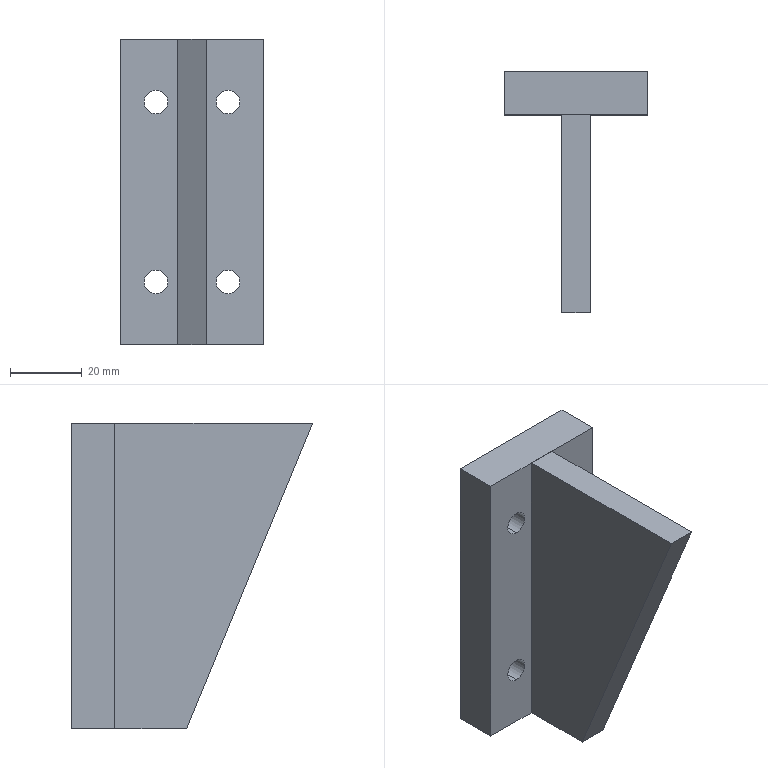Part | STEP file | 01-Positioning block seat | 2 solids | 20 faces | box 40 x 67 x 85 mm | volume 64658 mm3 | plane 12 | cylinder 8 | commonest cylinder face diameters 6.6 x8
STEP:
#1=CARTESIAN_POINT('',(0.,0.,0.));
#2=DIRECTION('',(0.,0.,1.));
#3=DIRECTION('',(1.,0.,0.));
#4=AXIS2_PLACEMENT_3D('',#1,#2,#3);
#5=CARTESIAN_POINT('',(-10.,0.,20.8));
#6=VERTEX_POINT('',#5);
#7=CARTESIAN_POINT('',(-10.,12.,20.8));
#8=VERTEX_POINT('',#7);
#9=CARTESIAN_POINT('',(-10.,27.,20.8));
#10=DIRECTION('',(0.,1.,0.));
#11=VECTOR('',#10,1.);
#12=LINE('',#9,#11);
#13=CARTESIAN_POINT('',(-10.,27.,17.5));
#14=DIRECTION('',(0.,1.,0.));
#15=DIRECTION('',(0.,0.,1.));
#16=AXIS2_PLACEMENT_3D('',#13,#14,#15);
#17=CYLINDRICAL_SURFACE('',#16,3.3);
#18=CARTESIAN_POINT('',(6.283,0.));
#19=DIRECTION('',(0.,1.));
#20=VECTOR('',#19,1.);
#21=LINE('',#18,#20);
#22=(GEOMETRIC_REPRESENTATION_CONTEXT(2)PARAMETRIC_REPRESENTATION_CONTEXT()REPRESENTATION_CONTEXT('',''));
#23=DEFINITIONAL_REPRESENTATION('',(#21),#22);
#24=PCURVE('',#17,#23);
#25=CARTESIAN_POINT('',(-10.,27.,17.5));
#26=DIRECTION('',(0.,1.,0.));
#27=DIRECTION('',(0.,0.,1.));
#28=AXIS2_PLACEMENT_3D('',#25,#26,#27);
#29=CYLINDRICAL_SURFACE('',#28,3.3);
#30=CARTESIAN_POINT('',(0.,0.));
#31=DIRECTION('',(0.,1.));
#32=VECTOR('',#31,1.);
#33=LINE('',#30,#32);
#34=(GEOMETRIC_REPRESENTATION_CONTEXT(2)PARAMETRIC_REPRESENTATION_CONTEXT()REPRESENTATION_CONTEXT('',''));
#35=DEFINITIONAL_REPRESENTATION('',(#33),#34);
#36=PCURVE('',#29,#35);
#37=SURFACE_CURVE('',#12,(#24,#36),.PCURVE_S1.);
#38=EDGE_CURVE('',#6,#8,#37,.T.);
#39=ORIENTED_EDGE('',*,*,#38,.T.);
#40=CARTESIAN_POINT('',(-10.,12.,14.2));
#41=VERTEX_POINT('',#40);
#42=CARTESIAN_POINT('',(-10.,12.,17.5));
#43=DIRECTION('',(0.,-1.,0.));
#44=DIRECTION('',(0.,0.,-1.));
#45=AXIS2_PLACEMENT_3D('',#42,#43,#44);
#46=CIRCLE('',#45,3.3);
#47=CARTESIAN_POINT('',(9.425,-15.));
#48=DIRECTION('',(-1.,0.));
#49=VECTOR('',#48,1.);
#50=LINE('',#47,#49);
#51=(GEOMETRIC_REPRESENTATION_CONTEXT(2)PARAMETRIC_REPRESENTATION_CONTEXT()REPRESENTATION_CONTEXT('',''));
#52=DEFINITIONAL_REPRESENTATION('',(#50),#51);
#53=PCURVE('',#17,#52);
#54=CARTESIAN_POINT('',(20.,12.,85.));
#55=DIRECTION('',(0.,-1.,0.));
#56=DIRECTION('',(0.,0.,-1.));
#57=AXIS2_PLACEMENT_3D('',#54,#55,#56);
#58=PLANE('',#57);
#59=CARTESIAN_POINT('',(67.5,-30.));
#60=DIRECTION('',(1.,0.));
#61=AXIS2_PLACEMENT_2D('',#59,#60);
#62=CIRCLE('',#61,3.3);
#63=(GEOMETRIC_REPRESENTATION_CONTEXT(2)PARAMETRIC_REPRESENTATION_CONTEXT()REPRESENTATION_CONTEXT('',''));
#64=DEFINITIONAL_REPRESENTATION('',(#62),#63);
#65=PCURVE('',#58,#64);
#66=SURFACE_CURVE('',#46,(#53,#65),.PCURVE_S1.);
#67=EDGE_CURVE('',#8,#41,#66,.T.);
#68=ORIENTED_EDGE('',*,*,#67,.T.);
#69=CARTESIAN_POINT('',(-10.,0.,14.2));
#70=VERTEX_POINT('',#69);
#71=CARTESIAN_POINT('',(-10.,27.,14.2));
#72=DIRECTION('',(0.,1.,0.));
#73=VECTOR('',#72,1.);
#74=LINE('',#71,#73);
#75=CARTESIAN_POINT('',(3.142,0.));
#76=DIRECTION('',(0.,1.));
#77=VECTOR('',#76,1.);
#78=LINE('',#75,#77);
#79=(GEOMETRIC_REPRESENTATION_CONTEXT(2)PARAMETRIC_REPRESENTATION_CONTEXT()REPRESENTATION_CONTEXT('',''));
#80=DEFINITIONAL_REPRESENTATION('',(#78),#79);
#81=PCURVE('',#17,#80);
#82=CARTESIAN_POINT('',(3.142,0.));
#83=DIRECTION('',(0.,1.));
#84=VECTOR('',#83,1.);
#85=LINE('',#82,#84);
#86=(GEOMETRIC_REPRESENTATION_CONTEXT(2)PARAMETRIC_REPRESENTATION_CONTEXT()REPRESENTATION_CONTEXT('',''));
#87=DEFINITIONAL_REPRESENTATION('',(#85),#86);
#88=PCURVE('',#29,#87);
#89=SURFACE_CURVE('',#74,(#81,#88),.PCURVE_S1.);
#90=EDGE_CURVE('',#70,#41,#89,.T.);
#91=ORIENTED_EDGE('',*,*,#90,.F.);
#92=CARTESIAN_POINT('',(-10.,0.,17.5));
#93=DIRECTION('',(0.,1.,0.));
#94=DIRECTION('',(0.,0.,1.));
#95=AXIS2_PLACEMENT_3D('',#92,#93,#94);
#96=CIRCLE('',#95,3.3);
#97=CARTESIAN_POINT('',(0.,-27.));
#98=DIRECTION('',(1.,0.));
#99=VECTOR('',#98,1.);
#100=LINE('',#97,#99);
#101=(GEOMETRIC_REPRESENTATION_CONTEXT(2)PARAMETRIC_REPRESENTATION_CONTEXT()REPRESENTATION_CONTEXT('',''));
#102=DEFINITIONAL_REPRESENTATION('',(#100),#101);
#103=PCURVE('',#17,#102);
#104=CARTESIAN_POINT('',(20.,0.,85.));
#105=DIRECTION('',(0.,1.,0.));
#106=DIRECTION('',(0.,0.,1.));
#107=AXIS2_PLACEMENT_3D('',#104,#105,#106);
#108=PLANE('',#107);
#109=CARTESIAN_POINT('',(-67.5,-30.));
#110=DIRECTION('',(1.,0.));
#111=AXIS2_PLACEMENT_2D('',#109,#110);
#112=CIRCLE('',#111,3.3);
#113=(GEOMETRIC_REPRESENTATION_CONTEXT(2)PARAMETRIC_REPRESENTATION_CONTEXT()REPRESENTATION_CONTEXT('',''));
#114=DEFINITIONAL_REPRESENTATION('',(#112),#113);
#115=PCURVE('',#108,#114);
#116=SURFACE_CURVE('',#96,(#103,#115),.PCURVE_S1.);
#117=EDGE_CURVE('',#70,#6,#116,.T.);
#118=ORIENTED_EDGE('',*,*,#117,.T.);
#119=EDGE_LOOP('',(#39,#68,#91,#118));
#120=FACE_BOUND('',#119,.F.);
#121=ADVANCED_FACE('',(#120),#17,.F.);
#122=CARTESIAN_POINT('',(-10.,0.,70.8));
#123=VERTEX_POINT('',#122);
#124=CARTESIAN_POINT('',(-10.,12.,70.8));
#125=VERTEX_POINT('',#124);
#126=CARTESIAN_POINT('',(-10.,27.,70.8));
#127=DIRECTION('',(0.,1.,0.));
#128=VECTOR('',#127,1.);
#129=LINE('',#126,#128);
#130=CARTESIAN_POINT('',(-10.,27.,67.5));
#131=DIRECTION('',(0.,1.,0.));
#132=DIRECTION('',(0.,0.,1.));
#133=AXIS2_PLACEMENT_3D('',#130,#131,#132);
#134=CYLINDRICAL_SURFACE('',#133,3.3);
#135=CARTESIAN_POINT('',(6.283,0.));
#136=DIRECTION('',(0.,1.));
#137=VECTOR('',#136,1.);
#138=LINE('',#135,#137);
#139=(GEOMETRIC_REPRESENTATION_CONTEXT(2)PARAMETRIC_REPRESENTATION_CONTEXT()REPRESENTATION_CONTEXT('',''));
#140=DEFINITIONAL_REPRESENTATION('',(#138),#139);
#141=PCURVE('',#134,#140);
#142=CARTESIAN_POINT('',(-10.,27.,67.5));
#143=DIRECTION('',(0.,1.,0.));
#144=DIRECTION('',(0.,0.,1.));
#145=AXIS2_PLACEMENT_3D('',#142,#143,#144);
#146=CYLINDRICAL_SURFACE('',#145,3.3);
#147=CARTESIAN_POINT('',(0.,0.));
#148=DIRECTION('',(0.,1.));
#149=VECTOR('',#148,1.);
#150=LINE('',#147,#149);
#151=(GEOMETRIC_REPRESENTATION_CONTEXT(2)PARAMETRIC_REPRESENTATION_CONTEXT()REPRESENTATION_CONTEXT('',''));
#152=DEFINITIONAL_REPRESENTATION('',(#150),#151);
#153=PCURVE('',#146,#152);
#154=SURFACE_CURVE('',#129,(#141,#153),.PCURVE_S1.);
#155=EDGE_CURVE('',#123,#125,#154,.T.);
#156=ORIENTED_EDGE('',*,*,#155,.T.);
#157=CARTESIAN_POINT('',(-10.,12.,64.2));
#158=VERTEX_POINT('',#157);
#159=CARTESIAN_POINT('',(-10.,12.,67.5));
#160=DIRECTION('',(0.,-1.,0.));
#161=DIRECTION('',(0.,0.,-1.));
#162=AXIS2_PLACEMENT_3D('',#159,#160,#161);
#163=CIRCLE('',#162,3.3);
#164=CARTESIAN_POINT('',(9.425,-15.));
#165=DIRECTION('',(-1.,0.));
#166=VECTOR('',#165,1.);
#167=LINE('',#164,#166);
#168=(GEOMETRIC_REPRESENTATION_CONTEXT(2)PARAMETRIC_REPRESENTATION_CONTEXT()REPRESENTATION_CONTEXT('',''));
#169=DEFINITIONAL_REPRESENTATION('',(#167),#168);
#170=PCURVE('',#134,#169);
#171=CARTESIAN_POINT('',(17.5,-30.));
#172=DIRECTION('',(1.,0.));
#173=AXIS2_PLACEMENT_2D('',#171,#172);
#174=CIRCLE('',#173,3.3);
#175=(GEOMETRIC_REPRESENTATION_CONTEXT(2)PARAMETRIC_REPRESENTATION_CONTEXT()REPRESENTATION_CONTEXT('',''));
#176=DEFINITIONAL_REPRESENTATION('',(#174),#175);
#177=PCURVE('',#58,#176);
#178=SURFACE_CURVE('',#163,(#170,#177),.PCURVE_S1.);
#179=EDGE_CURVE('',#125,#158,#178,.T.);
#180=ORIENTED_EDGE('',*,*,#179,.T.);
#181=CARTESIAN_POINT('',(-10.,0.,64.2));
#182=VERTEX_POINT('',#181);
#183=CARTESIAN_POINT('',(-10.,27.,64.2));
#184=DIRECTION('',(0.,1.,0.));
#185=VECTOR('',#184,1.);
#186=LINE('',#183,#185);
#187=CARTESIAN_POINT('',(3.142,0.));
#188=DIRECTION('',(0.,1.));
#189=VECTOR('',#188,1.);
#190=LINE('',#187,#189);
#191=(GEOMETRIC_REPRESENTATION_CONTEXT(2)PARAMETRIC_REPRESENTATION_CONTEXT()REPRESENTATION_CONTEXT('',''));
#192=DEFINITIONAL_REPRESENTATION('',(#190),#191);
#193=PCURVE('',#134,#192);
#194=CARTESIAN_POINT('',(3.142,0.));
#195=DIRECTION('',(0.,1.));
#196=VECTOR('',#195,1.);
#197=LINE('',#194,#196);
#198=(GEOMETRIC_REPRESENTATION_CONTEXT(2)PARAMETRIC_REPRESENTATION_CONTEXT()REPRESENTATION_CONTEXT('',''));
#199=DEFINITIONAL_REPRESENTATION('',(#197),#198);
#200=PCURVE('',#146,#199);
#201=SURFACE_CURVE('',#186,(#193,#200),.PCURVE_S1.);
#202=EDGE_CURVE('',#182,#158,#201,.T.);
#203=ORIENTED_EDGE('',*,*,#202,.F.);
#204=CARTESIAN_POINT('',(-10.,0.,67.5));
#205=DIRECTION('',(0.,1.,0.));
#206=DIRECTION('',(0.,0.,1.));
#207=AXIS2_PLACEMENT_3D('',#204,#205,#206);
#208=CIRCLE('',#207,3.3);
#209=CARTESIAN_POINT('',(0.,-27.));
#210=DIRECTION('',(1.,0.));
#211=VECTOR('',#210,1.);
#212=LINE('',#209,#211);
#213=(GEOMETRIC_REPRESENTATION_CONTEXT(2)PARAMETRIC_REPRESENTATION_CONTEXT()REPRESENTATION_CONTEXT('',''));
#214=DEFINITIONAL_REPRESENTATION('',(#212),#213);
#215=PCURVE('',#134,#214);
#216=CARTESIAN_POINT('',(-17.5,-30.));
#217=DIRECTION('',(1.,0.));
#218=AXIS2_PLACEMENT_2D('',#216,#217);
#219=CIRCLE('',#218,3.3);
#220=(GEOMETRIC_REPRESENTATION_CONTEXT(2)PARAMETRIC_REPRESENTATION_CONTEXT()REPRESENTATION_CONTEXT('',''));
#221=DEFINITIONAL_REPRESENTATION('',(#219),#220);
#222=PCURVE('',#108,#221);
#223=SURFACE_CURVE('',#208,(#215,#222),.PCURVE_S1.);
#224=EDGE_CURVE('',#182,#123,#223,.T.);
#225=ORIENTED_EDGE('',*,*,#224,.T.);
#226=EDGE_LOOP('',(#156,#180,#203,#225));
#227=FACE_BOUND('',#226,.F.);
#228=ADVANCED_FACE('',(#227),#134,.F.);
#229=CARTESIAN_POINT('',(10.,0.,20.8));
#230=VERTEX_POINT('',#229);
#231=CARTESIAN_POINT('',(10.,12.,20.8));
#232=VERTEX_POINT('',#231);
#233=CARTESIAN_POINT('',(10.,27.,20.8));
#234=DIRECTION('',(0.,1.,0.));
#235=VECTOR('',#234,1.);
#236=LINE('',#233,#235);
#237=CARTESIAN_POINT('',(10.,27.,17.5));
#238=DIRECTION('',(0.,1.,0.));
#239=DIRECTION('',(0.,0.,1.));
#240=AXIS2_PLACEMENT_3D('',#237,#238,#239);
#241=CYLINDRICAL_SURFACE('',#240,3.3);
#242=CARTESIAN_POINT('',(6.283,0.));
#243=DIRECTION('',(0.,1.));
#244=VECTOR('',#243,1.);
#245=LINE('',#242,#244);
#246=(GEOMETRIC_REPRESENTATION_CONTEXT(2)PARAMETRIC_REPRESENTATION_CONTEXT()REPRESENTATION_CONTEXT('',''));
#247=DEFINITIONAL_REPRESENTATION('',(#245),#246);
#248=PCURVE('',#241,#247);
#249=CARTESIAN_POINT('',(10.,27.,17.5));
#250=DIRECTION('',(0.,1.,0.));
#251=DIRECTION('',(0.,0.,1.));
#252=AXIS2_PLACEMENT_3D('',#249,#250,#251);
#253=CYLINDRICAL_SURFACE('',#252,3.3);
#254=CARTESIAN_POINT('',(0.,0.));
#255=DIRECTION('',(0.,1.));
#256=VECTOR('',#255,1.);
#257=LINE('',#254,#256);
#258=(GEOMETRIC_REPRESENTATION_CONTEXT(2)PARAMETRIC_REPRESENTATION_CONTEXT()REPRESENTATION_CONTEXT('',''));
#259=DEFINITIONAL_REPRESENTATION('',(#257),#258);
#260=PCURVE('',#253,#259);
#261=SURFACE_CURVE('',#236,(#248,#260),.PCURVE_S1.);
#262=EDGE_CURVE('',#230,#232,#261,.T.);
#263=ORIENTED_EDGE('',*,*,#262,.T.);
#264=CARTESIAN_POINT('',(10.,12.,14.2));
#265=VERTEX_POINT('',#264);
#266=CARTESIAN_POINT('',(10.,12.,17.5));
#267=DIRECTION('',(0.,-1.,0.));
#268=DIRECTION('',(0.,0.,-1.));
#269=AXIS2_PLACEMENT_3D('',#266,#267,#268);
#270=CIRCLE('',#269,3.3);
#271=CARTESIAN_POINT('',(9.425,-15.));
#272=DIRECTION('',(-1.,0.));
#273=VECTOR('',#272,1.);
#274=LINE('',#271,#273);
#275=(GEOMETRIC_REPRESENTATION_CONTEXT(2)PARAMETRIC_REPRESENTATION_CONTEXT()REPRESENTATION_CONTEXT('',''));
#276=DEFINITIONAL_REPRESENTATION('',(#274),#275);
#277=PCURVE('',#241,#276);
#278=CARTESIAN_POINT('',(67.5,-10.));
#279=DIRECTION('',(1.,0.));
#280=AXIS2_PLACEMENT_2D('',#278,#279);
#281=CIRCLE('',#280,3.3);
#282=(GEOMETRIC_REPRESENTATION_CONTEXT(2)PARAMETRIC_REPRESENTATION_CONTEXT()REPRESENTATION_CONTEXT('',''));
#283=DEFINITIONAL_REPRESENTATION('',(#281),#282);
#284=PCURVE('',#58,#283);
#285=SURFACE_CURVE('',#270,(#277,#284),.PCURVE_S1.);
#286=EDGE_CURVE('',#232,#265,#285,.T.);
#287=ORIENTED_EDGE('',*,*,#286,.T.);
#288=CARTESIAN_POINT('',(10.,0.,14.2));
#289=VERTEX_POINT('',#288);
#290=CARTESIAN_POINT('',(10.,27.,14.2));
#291=DIRECTION('',(0.,1.,0.));
#292=VECTOR('',#291,1.);
#293=LINE('',#290,#292);
#294=CARTESIAN_POINT('',(3.142,0.));
#295=DIRECTION('',(0.,1.));
#296=VECTOR('',#295,1.);
#297=LINE('',#294,#296);
#298=(GEOMETRIC_REPRESENTATION_CONTEXT(2)PARAMETRIC_REPRESENTATION_CONTEXT()REPRESENTATION_CONTEXT('',''));
#299=DEFINITIONAL_REPRESENTATION('',(#297),#298);
#300=PCURVE('',#241,#299);
#301=CARTESIAN_POINT('',(3.142,0.));
#302=DIRECTION('',(0.,1.));
#303=VECTOR('',#302,1.);
#304=LINE('',#301,#303);
#305=(GEOMETRIC_REPRESENTATION_CONTEXT(2)PARAMETRIC_REPRESENTATION_CONTEXT()REPRESENTATION_CONTEXT('',''));
#306=DEFINITIONAL_REPRESENTATION('',(#304),#305);
#307=PCURVE('',#253,#306);
#308=SURFACE_CURVE('',#293,(#300,#307),.PCURVE_S1.);
#309=EDGE_CURVE('',#289,#265,#308,.T.);
#310=ORIENTED_EDGE('',*,*,#309,.F.);
#311=CARTESIAN_POINT('',(10.,0.,17.5));
#312=DIRECTION('',(0.,1.,0.));
#313=DIRECTION('',(0.,0.,1.));
#314=AXIS2_PLACEMENT_3D('',#311,#312,#313);
#315=CIRCLE('',#314,3.3);
#316=CARTESIAN_POINT('',(0.,-27.));
#317=DIRECTION('',(1.,0.));
#318=VECTOR('',#317,1.);
#319=LINE('',#316,#318);
#320=(GEOMETRIC_REPRESENTATION_CONTEXT(2)PARAMETRIC_REPRESENTATION_CONTEXT()REPRESENTATION_CONTEXT('',''));
#321=DEFINITIONAL_REPRESENTATION('',(#319),#320);
#322=PCURVE('',#241,#321);
#323=CARTESIAN_POINT('',(-67.5,-10.));
#324=DIRECTION('',(1.,0.));
#325=AXIS2_PLACEMENT_2D('',#323,#324);
#326=CIRCLE('',#325,3.3);
#327=(GEOMETRIC_REPRESENTATION_CONTEXT(2)PARAMETRIC_REPRESENTATION_CONTEXT()REPRESENTATION_CONTEXT('',''));
#328=DEFINITIONAL_REPRESENTATION('',(#326),#327);
#329=PCURVE('',#108,#328);
#330=SURFACE_CURVE('',#315,(#322,#329),.PCURVE_S1.);
#331=EDGE_CURVE('',#289,#230,#330,.T.);
#332=ORIENTED_EDGE('',*,*,#331,.T.);
#333=EDGE_LOOP('',(#263,#287,#310,#332));
#334=FACE_BOUND('',#333,.F.);
#335=ADVANCED_FACE('',(#334),#241,.F.);
#336=CARTESIAN_POINT('',(10.,0.,70.8));
#337=VERTEX_POINT('',#336);
#338=CARTESIAN_POINT('',(10.,12.,70.8));
#339=VERTEX_POINT('',#338);
#340=CARTESIAN_POINT('',(10.,27.,70.8));
#341=DIRECTION('',(0.,1.,0.));
#342=VECTOR('',#341,1.);
#343=LINE('',#340,#342);
#344=CARTESIAN_POINT('',(10.,27.,67.5));
#345=DIRECTION('',(0.,1.,0.));
#346=DIRECTION('',(0.,0.,1.));
#347=AXIS2_PLACEMENT_3D('',#344,#345,#346);
#348=CYLINDRICAL_SURFACE('',#347,3.3);
#349=CARTESIAN_POINT('',(6.283,0.));
#350=DIRECTION('',(0.,1.));
#351=VECTOR('',#350,1.);
#352=LINE('',#349,#351);
#353=(GEOMETRIC_REPRESENTATION_CONTEXT(2)PARAMETRIC_REPRESENTATION_CONTEXT()REPRESENTATION_CONTEXT('',''));
#354=DEFINITIONAL_REPRESENTATION('',(#352),#353);
#355=PCURVE('',#348,#354);
#356=CARTESIAN_POINT('',(10.,27.,67.5));
#357=DIRECTION('',(0.,1.,0.));
#358=DIRECTION('',(0.,0.,1.));
#359=AXIS2_PLACEMENT_3D('',#356,#357,#358);
#360=CYLINDRICAL_SURFACE('',#359,3.3);
#361=CARTESIAN_POINT('',(0.,0.));
#362=DIRECTION('',(0.,1.));
#363=VECTOR('',#362,1.);
#364=LINE('',#361,#363);
#365=(GEOMETRIC_REPRESENTATION_CONTEXT(2)PARAMETRIC_REPRESENTATION_CONTEXT()REPRESENTATION_CONTEXT('',''));
#366=DEFINITIONAL_REPRESENTATION('',(#364),#365);
#367=PCURVE('',#360,#366);
#368=SURFACE_CURVE('',#343,(#355,#367),.PCURVE_S1.);
#369=EDGE_CURVE('',#337,#339,#368,.T.);
#370=ORIENTED_EDGE('',*,*,#369,.T.);
#371=CARTESIAN_POINT('',(10.,12.,64.2));
#372=VERTEX_POINT('',#371);
#373=CARTESIAN_POINT('',(10.,12.,67.5));
#374=DIRECTION('',(0.,-1.,0.));
#375=DIRECTION('',(0.,0.,-1.));
#376=AXIS2_PLACEMENT_3D('',#373,#374,#375);
#377=CIRCLE('',#376,3.3);
#378=CARTESIAN_POINT('',(9.425,-15.));
#379=DIRECTION('',(-1.,0.));
#380=VECTOR('',#379,1.);
#381=LINE('',#378,#380);
#382=(GEOMETRIC_REPRESENTATION_CONTEXT(2)PARAMETRIC_REPRESENTATION_CONTEXT()REPRESENTATION_CONTEXT('',''));
#383=DEFINITIONAL_REPRESENTATION('',(#381),#382);
#384=PCURVE('',#348,#383);
#385=CARTESIAN_POINT('',(17.5,-10.));
#386=DIRECTION('',(1.,0.));
#387=AXIS2_PLACEMENT_2D('',#385,#386);
#388=CIRCLE('',#387,3.3);
#389=(GEOMETRIC_REPRESENTATION_CONTEXT(2)PARAMETRIC_REPRESENTATION_CONTEXT()REPRESENTATION_CONTEXT('',''));
#390=DEFINITIONAL_REPRESENTATION('',(#388),#389);
#391=PCURVE('',#58,#390);
#392=SURFACE_CURVE('',#377,(#384,#391),.PCURVE_S1.);
#393=EDGE_CURVE('',#339,#372,#392,.T.);
#394=ORIENTED_EDGE('',*,*,#393,.T.);
#395=CARTESIAN_POINT('',(10.,0.,64.2));
#396=VERTEX_POINT('',#395);
#397=CARTESIAN_POINT('',(10.,27.,64.2));
#398=DIRECTION('',(0.,1.,0.));
#399=VECTOR('',#398,1.);
#400=LINE('',#397,#399);
#401=CARTESIAN_POINT('',(3.142,0.));
#402=DIRECTION('',(0.,1.));
#403=VECTOR('',#402,1.);
#404=LINE('',#401,#403);
#405=(GEOMETRIC_REPRESENTATION_CONTEXT(2)PARAMETRIC_REPRESENTATION_CONTEXT()REPRESENTATION_CONTEXT('',''));
#406=DEFINITIONAL_REPRESENTATION('',(#404),#405);
#407=PCURVE('',#348,#406);
#408=CARTESIAN_POINT('',(3.142,0.));
#409=DIRECTION('',(0.,1.));
#410=VECTOR('',#409,1.);
#411=LINE('',#408,#410);
#412=(GEOMETRIC_REPRESENTATION_CONTEXT(2)PARAMETRIC_REPRESENTATION_CONTEXT()REPRESENTATION_CONTEXT('',''));
#413=DEFINITIONAL_REPRESENTATION('',(#411),#412);
#414=PCURVE('',#360,#413);
#415=SURFACE_CURVE('',#400,(#407,#414),.PCURVE_S1.);
#416=EDGE_CURVE('',#396,#372,#415,.T.);
#417=ORIENTED_EDGE('',*,*,#416,.F.);
#418=CARTESIAN_POINT('',(10.,0.,67.5));
#419=DIRECTION('',(0.,1.,0.));
#420=DIRECTION('',(0.,0.,1.));
#421=AXIS2_PLACEMENT_3D('',#418,#419,#420);
#422=CIRCLE('',#421,3.3);
#423=CARTESIAN_POINT('',(0.,-27.));
#424=DIRECTION('',(1.,0.));
#425=VECTOR('',#424,1.);
#426=LINE('',#423,#425);
#427=(GEOMETRIC_REPRESENTATION_CONTEXT(2)PARAMETRIC_REPRESENTATION_CONTEXT()REPRESENTATION_CONTEXT('',''));
#428=DEFINITIONAL_REPRESENTATION('',(#426),#427);
#429=PCURVE('',#348,#428);
#430=CARTESIAN_POINT('',(-17.5,-10.));
#431=DIRECTION('',(1.,0.));
#432=AXIS2_PLACEMENT_2D('',#430,#431);
#433=CIRCLE('',#432,3.3);
#434=(GEOMETRIC_REPRESENTATION_CONTEXT(2)PARAMETRIC_REPRESENTATION_CONTEXT()REPRESENTATION_CONTEXT('',''));
#435=DEFINITIONAL_REPRESENTATION('',(#433),#434);
#436=PCURVE('',#108,#435);
#437=SURFACE_CURVE('',#422,(#429,#436),.PCURVE_S1.);
#438=EDGE_CURVE('',#396,#337,#437,.T.);
#439=ORIENTED_EDGE('',*,*,#438,.T.);
#440=EDGE_LOOP('',(#370,#394,#417,#439));
#441=FACE_BOUND('',#440,.F.);
#442=ADVANCED_FACE('',(#441),#348,.F.);
#443=CARTESIAN_POINT('',(-20.,12.,85.));
#444=VERTEX_POINT('',#443);
#445=CARTESIAN_POINT('',(-20.,0.,85.));
#446=VERTEX_POINT('',#445);
#447=CARTESIAN_POINT('',(-20.,0.,85.));
#448=DIRECTION('',(0.,-1.,0.));
#449=VECTOR('',#448,1.);
#450=LINE('',#447,#449);
#451=CARTESIAN_POINT('',(20.,0.,85.));
#452=DIRECTION('',(0.,0.,-1.));
#453=DIRECTION('',(-1.,0.,0.));
#454=AXIS2_PLACEMENT_3D('',#451,#452,#453);
#455=PLANE('',#454);
#456=CARTESIAN_POINT('',(40.,0.));
#457=DIRECTION('',(0.,-1.));
#458=VECTOR('',#457,1.);
#459=LINE('',#456,#458);
#460=(GEOMETRIC_REPRESENTATION_CONTEXT(2)PARAMETRIC_REPRESENTATION_CONTEXT()REPRESENTATION_CONTEXT('',''));
#461=DEFINITIONAL_REPRESENTATION('',(#459),#460);
#462=PCURVE('',#455,#461);
#463=CARTESIAN_POINT('',(-20.,0.,0.));
#464=DIRECTION('',(-1.,0.,0.));
#465=DIRECTION('',(0.,0.,1.));
#466=AXIS2_PLACEMENT_3D('',#463,#464,#465);
#467=PLANE('',#466);
#468=CARTESIAN_POINT('',(85.,0.));
#469=DIRECTION('',(0.,-1.));
#470=VECTOR('',#469,1.);
#471=LINE('',#468,#470);
#472=(GEOMETRIC_REPRESENTATION_CONTEXT(2)PARAMETRIC_REPRESENTATION_CONTEXT()REPRESENTATION_CONTEXT('',''));
#473=DEFINITIONAL_REPRESENTATION('',(#471),#472);
#474=PCURVE('',#467,#473);
#475=SURFACE_CURVE('',#450,(#462,#474),.PCURVE_S1.);
#476=EDGE_CURVE('',#444,#446,#475,.T.);
#477=ORIENTED_EDGE('',*,*,#476,.T.);
#478=CARTESIAN_POINT('',(20.,0.,85.));
#479=VERTEX_POINT('',#478);
#480=CARTESIAN_POINT('',(20.,0.,85.));
#481=DIRECTION('',(-1.,0.,0.));
#482=VECTOR('',#481,1.);
#483=LINE('',#480,#482);
#484=CARTESIAN_POINT('',(0.,0.));
#485=DIRECTION('',(1.,0.));
#486=VECTOR('',#485,1.);
#487=LINE('',#484,#486);
#488=(GEOMETRIC_REPRESENTATION_CONTEXT(2)PARAMETRIC_REPRESENTATION_CONTEXT()REPRESENTATION_CONTEXT('',''));
#489=DEFINITIONAL_REPRESENTATION('',(#487),#488);
#490=PCURVE('',#455,#489);
#491=CARTESIAN_POINT('',(0.,0.));
#492=DIRECTION('',(0.,-1.));
#493=VECTOR('',#492,1.);
#494=LINE('',#491,#493);
#495=(GEOMETRIC_REPRESENTATION_CONTEXT(2)PARAMETRIC_REPRESENTATION_CONTEXT()REPRESENTATION_CONTEXT('',''));
#496=DEFINITIONAL_REPRESENTATION('',(#494),#495);
#497=PCURVE('',#108,#496);
#498=SURFACE_CURVE('',#483,(#490,#497),.PCURVE_S1.);
#499=EDGE_CURVE('',#479,#446,#498,.T.);
#500=ORIENTED_EDGE('',*,*,#499,.F.);
#501=CARTESIAN_POINT('',(20.,12.,85.));
#502=VERTEX_POINT('',#501);
#503=CARTESIAN_POINT('',(20.,0.,85.));
#504=DIRECTION('',(0.,-1.,0.));
#505=VECTOR('',#504,1.);
#506=LINE('',#503,#505);
#507=CARTESIAN_POINT('',(0.,0.));
#508=DIRECTION('',(0.,-1.));
#509=VECTOR('',#508,1.);
#510=LINE('',#507,#509);
#511=(GEOMETRIC_REPRESENTATION_CONTEXT(2)PARAMETRIC_REPRESENTATION_CONTEXT()REPRESENTATION_CONTEXT('',''));
#512=DEFINITIONAL_REPRESENTATION('',(#510),#511);
#513=PCURVE('',#455,#512);
#514=CARTESIAN_POINT('',(20.,0.,0.));
#515=DIRECTION('',(-1.,0.,0.));
#516=DIRECTION('',(0.,0.,1.));
#517=AXIS2_PLACEMENT_3D('',#514,#515,#516);
#518=PLANE('',#517);
#519=CARTESIAN_POINT('',(85.,0.));
#520=DIRECTION('',(0.,-1.));
#521=VECTOR('',#520,1.);
#522=LINE('',#519,#521);
#523=(GEOMETRIC_REPRESENTATION_CONTEXT(2)PARAMETRIC_REPRESENTATION_CONTEXT()REPRESENTATION_CONTEXT('',''));
#524=DEFINITIONAL_REPRESENTATION('',(#522),#523);
#525=PCURVE('',#518,#524);
#526=SURFACE_CURVE('',#506,(#513,#525),.PCURVE_S1.);
#527=EDGE_CURVE('',#502,#479,#526,.T.);
#528=ORIENTED_EDGE('',*,*,#527,.F.);
#529=CARTESIAN_POINT('',(20.,12.,85.));
#530=DIRECTION('',(-1.,0.,0.));
#531=VECTOR('',#530,1.);
#532=LINE('',#529,#531);
#533=CARTESIAN_POINT('',(0.,12.));
#534=DIRECTION('',(1.,0.));
#535=VECTOR('',#534,1.);
#536=LINE('',#533,#535);
#537=(GEOMETRIC_REPRESENTATION_CONTEXT(2)PARAMETRIC_REPRESENTATION_CONTEXT()REPRESENTATION_CONTEXT('',''));
#538=DEFINITIONAL_REPRESENTATION('',(#536),#537);
#539=PCURVE('',#455,#538);
#540=CARTESIAN_POINT('',(0.,0.));
#541=DIRECTION('',(0.,-1.));
#542=VECTOR('',#541,1.);
#543=LINE('',#540,#542);
#544=(GEOMETRIC_REPRESENTATION_CONTEXT(2)PARAMETRIC_REPRESENTATION_CONTEXT()REPRESENTATION_CONTEXT('',''));
#545=DEFINITIONAL_REPRESENTATION('',(#543),#544);
#546=PCURVE('',#58,#545);
#547=SURFACE_CURVE('',#532,(#539,#546),.PCURVE_S1.);
#548=EDGE_CURVE('',#502,#444,#547,.T.);
#549=ORIENTED_EDGE('',*,*,#548,.T.);
#550=EDGE_LOOP('',(#477,#500,#528,#549));
#551=FACE_BOUND('',#550,.T.);
#552=ADVANCED_FACE('',(#551),#455,.F.);
#553=CARTESIAN_POINT('',(-10.,0.,17.5));
#554=DIRECTION('',(0.,1.,0.));
#555=DIRECTION('',(0.,0.,1.));
#556=AXIS2_PLACEMENT_3D('',#553,#554,#555);
#557=CIRCLE('',#556,3.3);
#558=CARTESIAN_POINT('',(-67.5,-30.));
#559=DIRECTION('',(1.,0.));
#560=AXIS2_PLACEMENT_2D('',#558,#559);
#561=CIRCLE('',#560,3.3);
#562=(GEOMETRIC_REPRESENTATION_CONTEXT(2)PARAMETRIC_REPRESENTATION_CONTEXT()REPRESENTATION_CONTEXT('',''));
#563=DEFINITIONAL_REPRESENTATION('',(#561),#562);
#564=PCURVE('',#108,#563);
#565=CARTESIAN_POINT('',(0.,-27.));
#566=DIRECTION('',(1.,0.));
#567=VECTOR('',#566,1.);
#568=LINE('',#565,#567);
#569=(GEOMETRIC_REPRESENTATION_CONTEXT(2)PARAMETRIC_REPRESENTATION_CONTEXT()REPRESENTATION_CONTEXT('',''));
#570=DEFINITIONAL_REPRESENTATION('',(#568),#569);
#571=PCURVE('',#29,#570);
#572=SURFACE_CURVE('',#557,(#564,#571),.PCURVE_S1.);
#573=EDGE_CURVE('',#6,#70,#572,.T.);
#574=ORIENTED_EDGE('',*,*,#573,.T.);
#575=ORIENTED_EDGE('',*,*,#117,.T.);
#576=EDGE_LOOP('',(#574,#575));
#577=FACE_BOUND('',#576,.T.);
#578=CARTESIAN_POINT('',(-10.,0.,67.5));
#579=DIRECTION('',(0.,1.,0.));
#580=DIRECTION('',(0.,0.,1.));
#581=AXIS2_PLACEMENT_3D('',#578,#579,#580);
#582=CIRCLE('',#581,3.3);
#583=CARTESIAN_POINT('',(-17.5,-30.));
#584=DIRECTION('',(1.,0.));
#585=AXIS2_PLACEMENT_2D('',#583,#584);
#586=CIRCLE('',#585,3.3);
#587=(GEOMETRIC_REPRESENTATION_CONTEXT(2)PARAMETRIC_REPRESENTATION_CONTEXT()REPRESENTATION_CONTEXT('',''));
#588=DEFINITIONAL_REPRESENTATION('',(#586),#587);
#589=PCURVE('',#108,#588);
#590=CARTESIAN_POINT('',(0.,-27.));
#591=DIRECTION('',(1.,0.));
#592=VECTOR('',#591,1.);
#593=LINE('',#590,#592);
#594=(GEOMETRIC_REPRESENTATION_CONTEXT(2)PARAMETRIC_REPRESENTATION_CONTEXT()REPRESENTATION_CONTEXT('',''));
#595=DEFINITIONAL_REPRESENTATION('',(#593),#594);
#596=PCURVE('',#146,#595);
#597=SURFACE_CURVE('',#582,(#589,#596),.PCURVE_S1.);
#598=EDGE_CURVE('',#123,#182,#597,.T.);
#599=ORIENTED_EDGE('',*,*,#598,.T.);
#600=ORIENTED_EDGE('',*,*,#224,.T.);
#601=EDGE_LOOP('',(#599,#600));
#602=FACE_BOUND('',#601,.T.);
#603=CARTESIAN_POINT('',(10.,0.,17.5));
#604=DIRECTION('',(0.,1.,0.));
#605=DIRECTION('',(0.,0.,1.));
#606=AXIS2_PLACEMENT_3D('',#603,#604,#605);
#607=CIRCLE('',#606,3.3);
#608=CARTESIAN_POINT('',(-67.5,-10.));
#609=DIRECTION('',(1.,0.));
#610=AXIS2_PLACEMENT_2D('',#608,#609);
#611=CIRCLE('',#610,3.3);
#612=(GEOMETRIC_REPRESENTATION_CONTEXT(2)PARAMETRIC_REPRESENTATION_CONTEXT()REPRESENTATION_CONTEXT('',''));
#613=DEFINITIONAL_REPRESENTATION('',(#611),#612);
#614=PCURVE('',#108,#613);
#615=CARTESIAN_POINT('',(0.,-27.));
#616=DIRECTION('',(1.,0.));
#617=VECTOR('',#616,1.);
#618=LINE('',#615,#617);
#619=(GEOMETRIC_REPRESENTATION_CONTEXT(2)PARAMETRIC_REPRESENTATION_CONTEXT()REPRESENTATION_CONTEXT('',''));
#620=DEFINITIONAL_REPRESENTATION('',(#618),#619);
#621=PCURVE('',#253,#620);
#622=SURFACE_CURVE('',#607,(#614,#621),.PCURVE_S1.);
#623=EDGE_CURVE('',#230,#289,#622,.T.);
#624=ORIENTED_EDGE('',*,*,#623,.T.);
#625=ORIENTED_EDGE('',*,*,#331,.T.);
#626=EDGE_LOOP('',(#624,#625));
#627=FACE_BOUND('',#626,.T.);
#628=CARTESIAN_POINT('',(10.,0.,67.5));
#629=DIRECTION('',(0.,1.,0.));
#630=DIRECTION('',(0.,0.,1.));
#631=AXIS2_PLACEMENT_3D('',#628,#629,#630);
#632=CIRCLE('',#631,3.3);
#633=CARTESIAN_POINT('',(-17.5,-10.));
#634=DIRECTION('',(1.,0.));
#635=AXIS2_PLACEMENT_2D('',#633,#634);
#636=CIRCLE('',#635,3.3);
#637=(GEOMETRIC_REPRESENTATION_CONTEXT(2)PARAMETRIC_REPRESENTATION_CONTEXT()REPRESENTATION_CONTEXT('',''));
#638=DEFINITIONAL_REPRESENTATION('',(#636),#637);
#639=PCURVE('',#108,#638);
#640=CARTESIAN_POINT('',(0.,-27.));
#641=DIRECTION('',(1.,0.));
#642=VECTOR('',#641,1.);
#643=LINE('',#640,#642);
#644=(GEOMETRIC_REPRESENTATION_CONTEXT(2)PARAMETRIC_REPRESENTATION_CONTEXT()REPRESENTATION_CONTEXT('',''));
#645=DEFINITIONAL_REPRESENTATION('',(#643),#644);
#646=PCURVE('',#360,#645);
#647=SURFACE_CURVE('',#632,(#639,#646),.PCURVE_S1.);
#648=EDGE_CURVE('',#337,#396,#647,.T.);
#649=ORIENTED_EDGE('',*,*,#648,.T.);
#650=ORIENTED_EDGE('',*,*,#438,.T.);
#651=EDGE_LOOP('',(#649,#650));
#652=FACE_BOUND('',#651,.T.);
#653=CARTESIAN_POINT('',(-20.,0.,0.));
#654=VERTEX_POINT('',#653);
#655=CARTESIAN_POINT('',(-20.,0.,85.));
#656=DIRECTION('',(0.,0.,-1.));
#657=VECTOR('',#656,1.);
#658=LINE('',#655,#657);
#659=CARTESIAN_POINT('',(0.,-40.));
#660=DIRECTION('',(-1.,0.));
#661=VECTOR('',#660,1.);
#662=LINE('',#659,#661);
#663=(GEOMETRIC_REPRESENTATION_CONTEXT(2)PARAMETRIC_REPRESENTATION_CONTEXT()REPRESENTATION_CONTEXT('',''));
#664=DEFINITIONAL_REPRESENTATION('',(#662),#663);
#665=PCURVE('',#108,#664);
#666=CARTESIAN_POINT('',(85.,0.));
#667=DIRECTION('',(-1.,0.));
#668=VECTOR('',#667,1.);
#669=LINE('',#666,#668);
#670=(GEOMETRIC_REPRESENTATION_CONTEXT(2)PARAMETRIC_REPRESENTATION_CONTEXT()REPRESENTATION_CONTEXT('',''));
#671=DEFINITIONAL_REPRESENTATION('',(#669),#670);
#672=PCURVE('',#467,#671);
#673=SURFACE_CURVE('',#658,(#665,#672),.PCURVE_S1.);
#674=EDGE_CURVE('',#446,#654,#673,.T.);
#675=ORIENTED_EDGE('',*,*,#674,.T.);
#676=CARTESIAN_POINT('',(20.,0.,0.));
#677=VERTEX_POINT('',#676);
#678=CARTESIAN_POINT('',(20.,0.,0.));
#679=DIRECTION('',(-1.,0.,0.));
#680=VECTOR('',#679,1.);
#681=LINE('',#678,#680);
#682=CARTESIAN_POINT('',(-85.,0.));
#683=DIRECTION('',(0.,-1.));
#684=VECTOR('',#683,1.);
#685=LINE('',#682,#684);
#686=(GEOMETRIC_REPRESENTATION_CONTEXT(2)PARAMETRIC_REPRESENTATION_CONTEXT()REPRESENTATION_CONTEXT('',''));
#687=DEFINITIONAL_REPRESENTATION('',(#685),#686);
#688=PCURVE('',#108,#687);
#689=CARTESIAN_POINT('',(20.,0.,0.));
#690=DIRECTION('',(0.,0.,1.));
#691=DIRECTION('',(1.,0.,0.));
#692=AXIS2_PLACEMENT_3D('',#689,#690,#691);
#693=PLANE('',#692);
#694=CARTESIAN_POINT('',(0.,0.));
#695=DIRECTION('',(-1.,0.));
#696=VECTOR('',#695,1.);
#697=LINE('',#694,#696);
#698=(GEOMETRIC_REPRESENTATION_CONTEXT(2)PARAMETRIC_REPRESENTATION_CONTEXT()REPRESENTATION_CONTEXT('',''));
#699=DEFINITIONAL_REPRESENTATION('',(#697),#698);
#700=PCURVE('',#693,#699);
#701=SURFACE_CURVE('',#681,(#688,#700),.PCURVE_S1.);
#702=EDGE_CURVE('',#677,#654,#701,.T.);
#703=ORIENTED_EDGE('',*,*,#702,.F.);
#704=CARTESIAN_POINT('',(20.,0.,85.));
#705=DIRECTION('',(0.,0.,-1.));
#706=VECTOR('',#705,1.);
#707=LINE('',#704,#706);
#708=CARTESIAN_POINT('',(0.,0.));
#709=DIRECTION('',(-1.,0.));
#710=VECTOR('',#709,1.);
#711=LINE('',#708,#710);
#712=(GEOMETRIC_REPRESENTATION_CONTEXT(2)PARAMETRIC_REPRESENTATION_CONTEXT()REPRESENTATION_CONTEXT('',''));
#713=DEFINITIONAL_REPRESENTATION('',(#711),#712);
#714=PCURVE('',#108,#713);
#715=CARTESIAN_POINT('',(85.,0.));
#716=DIRECTION('',(-1.,0.));
#717=VECTOR('',#716,1.);
#718=LINE('',#715,#717);
#719=(GEOMETRIC_REPRESENTATION_CONTEXT(2)PARAMETRIC_REPRESENTATION_CONTEXT()REPRESENTATION_CONTEXT('',''));
#720=DEFINITIONAL_REPRESENTATION('',(#718),#719);
#721=PCURVE('',#518,#720);
#722=SURFACE_CURVE('',#707,(#714,#721),.PCURVE_S1.);
#723=EDGE_CURVE('',#479,#677,#722,.T.);
#724=ORIENTED_EDGE('',*,*,#723,.F.);
#725=ORIENTED_EDGE('',*,*,#499,.T.);
#726=EDGE_LOOP('',(#675,#703,#724,#725));
#727=FACE_BOUND('',#726,.T.);
#728=ADVANCED_FACE('',(#577,#602,#627,#652,#727),#108,.F.);
#729=CARTESIAN_POINT('',(-20.,12.,0.));
#730=VERTEX_POINT('',#729);
#731=CARTESIAN_POINT('',(-20.,0.,0.));
#732=DIRECTION('',(0.,1.,0.));
#733=VECTOR('',#732,1.);
#734=LINE('',#731,#733);
#735=CARTESIAN_POINT('',(-40.,0.));
#736=DIRECTION('',(0.,1.));
#737=VECTOR('',#736,1.);
#738=LINE('',#735,#737);
#739=(GEOMETRIC_REPRESENTATION_CONTEXT(2)PARAMETRIC_REPRESENTATION_CONTEXT()REPRESENTATION_CONTEXT('',''));
#740=DEFINITIONAL_REPRESENTATION('',(#738),#739);
#741=PCURVE('',#693,#740);
#742=CARTESIAN_POINT('',(0.,0.));
#743=DIRECTION('',(0.,1.));
#744=VECTOR('',#743,1.);
#745=LINE('',#742,#744);
#746=(GEOMETRIC_REPRESENTATION_CONTEXT(2)PARAMETRIC_REPRESENTATION_CONTEXT()REPRESENTATION_CONTEXT('',''));
#747=DEFINITIONAL_REPRESENTATION('',(#745),#746);
#748=PCURVE('',#467,#747);
#749=SURFACE_CURVE('',#734,(#741,#748),.PCURVE_S1.);
#750=EDGE_CURVE('',#654,#730,#749,.T.);
#751=ORIENTED_EDGE('',*,*,#750,.T.);
#752=CARTESIAN_POINT('',(20.,12.,0.));
#753=VERTEX_POINT('',#752);
#754=CARTESIAN_POINT('',(20.,12.,0.));
#755=DIRECTION('',(-1.,0.,0.));
#756=VECTOR('',#755,1.);
#757=LINE('',#754,#756);
#758=CARTESIAN_POINT('',(0.,12.));
#759=DIRECTION('',(-1.,0.));
#760=VECTOR('',#759,1.);
#761=LINE('',#758,#760);
#762=(GEOMETRIC_REPRESENTATION_CONTEXT(2)PARAMETRIC_REPRESENTATION_CONTEXT()REPRESENTATION_CONTEXT('',''));
#763=DEFINITIONAL_REPRESENTATION('',(#761),#762);
#764=PCURVE('',#693,#763);
#765=CARTESIAN_POINT('',(85.,0.));
#766=DIRECTION('',(0.,-1.));
#767=VECTOR('',#766,1.);
#768=LINE('',#765,#767);
#769=(GEOMETRIC_REPRESENTATION_CONTEXT(2)PARAMETRIC_REPRESENTATION_CONTEXT()REPRESENTATION_CONTEXT('',''));
#770=DEFINITIONAL_REPRESENTATION('',(#768),#769);
#771=PCURVE('',#58,#770);
#772=SURFACE_CURVE('',#757,(#764,#771),.PCURVE_S1.);
#773=EDGE_CURVE('',#753,#730,#772,.T.);
#774=ORIENTED_EDGE('',*,*,#773,.F.);
#775=CARTESIAN_POINT('',(20.,0.,0.));
#776=DIRECTION('',(0.,1.,0.));
#777=VECTOR('',#776,1.);
#778=LINE('',#775,#777);
#779=CARTESIAN_POINT('',(0.,0.));
#780=DIRECTION('',(0.,1.));
#781=VECTOR('',#780,1.);
#782=LINE('',#779,#781);
#783=(GEOMETRIC_REPRESENTATION_CONTEXT(2)PARAMETRIC_REPRESENTATION_CONTEXT()REPRESENTATION_CONTEXT('',''));
#784=DEFINITIONAL_REPRESENTATION('',(#782),#783);
#785=PCURVE('',#693,#784);
#786=CARTESIAN_POINT('',(0.,0.));
#787=DIRECTION('',(0.,1.));
#788=VECTOR('',#787,1.);
#789=LINE('',#786,#788);
#790=(GEOMETRIC_REPRESENTATION_CONTEXT(2)PARAMETRIC_REPRESENTATION_CONTEXT()REPRESENTATION_CONTEXT('',''));
#791=DEFINITIONAL_REPRESENTATION('',(#789),#790);
#792=PCURVE('',#518,#791);
#793=SURFACE_CURVE('',#778,(#785,#792),.PCURVE_S1.);
#794=EDGE_CURVE('',#677,#753,#793,.T.);
#795=ORIENTED_EDGE('',*,*,#794,.F.);
#796=ORIENTED_EDGE('',*,*,#702,.T.);
#797=EDGE_LOOP('',(#751,#774,#795,#796));
#798=FACE_BOUND('',#797,.T.);
#799=ADVANCED_FACE('',(#798),#693,.F.);
#800=ORIENTED_EDGE('',*,*,#67,.T.);
#801=CARTESIAN_POINT('',(-10.,12.,17.5));
#802=DIRECTION('',(0.,-1.,0.));
#803=DIRECTION('',(0.,0.,-1.));
#804=AXIS2_PLACEMENT_3D('',#801,#802,#803);
#805=CIRCLE('',#804,3.3);
#806=CARTESIAN_POINT('',(67.5,-30.));
#807=DIRECTION('',(1.,0.));
#808=AXIS2_PLACEMENT_2D('',#806,#807);
#809=CIRCLE('',#808,3.3);
#810=(GEOMETRIC_REPRESENTATION_CONTEXT(2)PARAMETRIC_REPRESENTATION_CONTEXT()REPRESENTATION_CONTEXT('',''));
#811=DEFINITIONAL_REPRESENTATION('',(#809),#810);
#812=PCURVE('',#58,#811);
#813=CARTESIAN_POINT('',(3.142,-15.));
#814=DIRECTION('',(-1.,0.));
#815=VECTOR('',#814,1.);
#816=LINE('',#813,#815);
#817=(GEOMETRIC_REPRESENTATION_CONTEXT(2)PARAMETRIC_REPRESENTATION_CONTEXT()REPRESENTATION_CONTEXT('',''));
#818=DEFINITIONAL_REPRESENTATION('',(#816),#817);
#819=PCURVE('',#29,#818);
#820=SURFACE_CURVE('',#805,(#812,#819),.PCURVE_S1.);
#821=EDGE_CURVE('',#41,#8,#820,.T.);
#822=ORIENTED_EDGE('',*,*,#821,.T.);
#823=EDGE_LOOP('',(#800,#822));
#824=FACE_BOUND('',#823,.T.);
#825=ORIENTED_EDGE('',*,*,#179,.T.);
#826=CARTESIAN_POINT('',(-10.,12.,67.5));
#827=DIRECTION('',(0.,-1.,0.));
#828=DIRECTION('',(0.,0.,-1.));
#829=AXIS2_PLACEMENT_3D('',#826,#827,#828);
#830=CIRCLE('',#829,3.3);
#831=CARTESIAN_POINT('',(17.5,-30.));
#832=DIRECTION('',(1.,0.));
#833=AXIS2_PLACEMENT_2D('',#831,#832);
#834=CIRCLE('',#833,3.3);
#835=(GEOMETRIC_REPRESENTATION_CONTEXT(2)PARAMETRIC_REPRESENTATION_CONTEXT()REPRESENTATION_CONTEXT('',''));
#836=DEFINITIONAL_REPRESENTATION('',(#834),#835);
#837=PCURVE('',#58,#836);
#838=CARTESIAN_POINT('',(3.142,-15.));
#839=DIRECTION('',(-1.,0.));
#840=VECTOR('',#839,1.);
#841=LINE('',#838,#840);
#842=(GEOMETRIC_REPRESENTATION_CONTEXT(2)PARAMETRIC_REPRESENTATION_CONTEXT()REPRESENTATION_CONTEXT('',''));
#843=DEFINITIONAL_REPRESENTATION('',(#841),#842);
#844=PCURVE('',#146,#843);
#845=SURFACE_CURVE('',#830,(#837,#844),.PCURVE_S1.);
#846=EDGE_CURVE('',#158,#125,#845,.T.);
#847=ORIENTED_EDGE('',*,*,#846,.T.);
#848=EDGE_LOOP('',(#825,#847));
#849=FACE_BOUND('',#848,.T.);
#850=ORIENTED_EDGE('',*,*,#286,.T.);
#851=CARTESIAN_POINT('',(10.,12.,17.5));
#852=DIRECTION('',(0.,-1.,0.));
#853=DIRECTION('',(0.,0.,-1.));
#854=AXIS2_PLACEMENT_3D('',#851,#852,#853);
#855=CIRCLE('',#854,3.3);
#856=CARTESIAN_POINT('',(67.5,-10.));
#857=DIRECTION('',(1.,0.));
#858=AXIS2_PLACEMENT_2D('',#856,#857);
#859=CIRCLE('',#858,3.3);
#860=(GEOMETRIC_REPRESENTATION_CONTEXT(2)PARAMETRIC_REPRESENTATION_CONTEXT()REPRESENTATION_CONTEXT('',''));
#861=DEFINITIONAL_REPRESENTATION('',(#859),#860);
#862=PCURVE('',#58,#861);
#863=CARTESIAN_POINT('',(3.142,-15.));
#864=DIRECTION('',(-1.,0.));
#865=VECTOR('',#864,1.);
#866=LINE('',#863,#865);
#867=(GEOMETRIC_REPRESENTATION_CONTEXT(2)PARAMETRIC_REPRESENTATION_CONTEXT()REPRESENTATION_CONTEXT('',''));
#868=DEFINITIONAL_REPRESENTATION('',(#866),#867);
#869=PCURVE('',#253,#868);
#870=SURFACE_CURVE('',#855,(#862,#869),.PCURVE_S1.);
#871=EDGE_CURVE('',#265,#232,#870,.T.);
#872=ORIENTED_EDGE('',*,*,#871,.T.);
#873=EDGE_LOOP('',(#850,#872));
#874=FACE_BOUND('',#873,.T.);
#875=ORIENTED_EDGE('',*,*,#393,.T.);
#876=CARTESIAN_POINT('',(10.,12.,67.5));
#877=DIRECTION('',(0.,-1.,0.));
#878=DIRECTION('',(0.,0.,-1.));
#879=AXIS2_PLACEMENT_3D('',#876,#877,#878);
#880=CIRCLE('',#879,3.3);
#881=CARTESIAN_POINT('',(17.5,-10.));
#882=DIRECTION('',(1.,0.));
#883=AXIS2_PLACEMENT_2D('',#881,#882);
#884=CIRCLE('',#883,3.3);
#885=(GEOMETRIC_REPRESENTATION_CONTEXT(2)PARAMETRIC_REPRESENTATION_CONTEXT()REPRESENTATION_CONTEXT('',''));
#886=DEFINITIONAL_REPRESENTATION('',(#884),#885);
#887=PCURVE('',#58,#886);
#888=CARTESIAN_POINT('',(3.142,-15.));
#889=DIRECTION('',(-1.,0.));
#890=VECTOR('',#889,1.);
#891=LINE('',#888,#890);
#892=(GEOMETRIC_REPRESENTATION_CONTEXT(2)PARAMETRIC_REPRESENTATION_CONTEXT()REPRESENTATION_CONTEXT('',''));
#893=DEFINITIONAL_REPRESENTATION('',(#891),#892);
#894=PCURVE('',#360,#893);
#895=SURFACE_CURVE('',#880,(#887,#894),.PCURVE_S1.);
#896=EDGE_CURVE('',#372,#339,#895,.T.);
#897=ORIENTED_EDGE('',*,*,#896,.T.);
#898=EDGE_LOOP('',(#875,#897));
#899=FACE_BOUND('',#898,.T.);
#900=CARTESIAN_POINT('',(-20.,12.,85.));
#901=DIRECTION('',(0.,0.,1.));
#902=VECTOR('',#901,1.);
#903=LINE('',#900,#902);
#904=CARTESIAN_POINT('',(0.,-40.));
#905=DIRECTION('',(-1.,0.));
#906=VECTOR('',#905,1.);
#907=LINE('',#904,#906);
#908=(GEOMETRIC_REPRESENTATION_CONTEXT(2)PARAMETRIC_REPRESENTATION_CONTEXT()REPRESENTATION_CONTEXT('',''));
#909=DEFINITIONAL_REPRESENTATION('',(#907),#908);
#910=PCURVE('',#58,#909);
#911=CARTESIAN_POINT('',(85.,12.));
#912=DIRECTION('',(1.,0.));
#913=VECTOR('',#912,1.);
#914=LINE('',#911,#913);
#915=(GEOMETRIC_REPRESENTATION_CONTEXT(2)PARAMETRIC_REPRESENTATION_CONTEXT()REPRESENTATION_CONTEXT('',''));
#916=DEFINITIONAL_REPRESENTATION('',(#914),#915);
#917=PCURVE('',#467,#916);
#918=SURFACE_CURVE('',#903,(#910,#917),.PCURVE_S1.);
#919=EDGE_CURVE('',#730,#444,#918,.T.);
#920=ORIENTED_EDGE('',*,*,#919,.T.);
#921=ORIENTED_EDGE('',*,*,#548,.F.);
#922=CARTESIAN_POINT('',(20.,12.,85.));
#923=DIRECTION('',(0.,0.,1.));
#924=VECTOR('',#923,1.);
#925=LINE('',#922,#924);
#926=CARTESIAN_POINT('',(0.,0.));
#927=DIRECTION('',(-1.,0.));
#928=VECTOR('',#927,1.);
#929=LINE('',#926,#928);
#930=(GEOMETRIC_REPRESENTATION_CONTEXT(2)PARAMETRIC_REPRESENTATION_CONTEXT()REPRESENTATION_CONTEXT('',''));
#931=DEFINITIONAL_REPRESENTATION('',(#929),#930);
#932=PCURVE('',#58,#931);
#933=CARTESIAN_POINT('',(85.,12.));
#934=DIRECTION('',(1.,0.));
#935=VECTOR('',#934,1.);
#936=LINE('',#933,#935);
#937=(GEOMETRIC_REPRESENTATION_CONTEXT(2)PARAMETRIC_REPRESENTATION_CONTEXT()REPRESENTATION_CONTEXT('',''));
#938=DEFINITIONAL_REPRESENTATION('',(#936),#937);
#939=PCURVE('',#518,#938);
#940=SURFACE_CURVE('',#925,(#932,#939),.PCURVE_S1.);
#941=EDGE_CURVE('',#753,#502,#940,.T.);
#942=ORIENTED_EDGE('',*,*,#941,.F.);
#943=ORIENTED_EDGE('',*,*,#773,.T.);
#944=EDGE_LOOP('',(#920,#921,#942,#943));
#945=FACE_BOUND('',#944,.T.);
#946=ADVANCED_FACE('',(#824,#849,#874,#899,#945),#58,.F.);
#947=ORIENTED_EDGE('',*,*,#527,.T.);
#948=ORIENTED_EDGE('',*,*,#723,.T.);
#949=ORIENTED_EDGE('',*,*,#794,.T.);
#950=ORIENTED_EDGE('',*,*,#941,.T.);
#951=EDGE_LOOP('',(#947,#948,#949,#950));
#952=FACE_BOUND('',#951,.T.);
#953=ADVANCED_FACE('',(#952),#518,.F.);
#954=ORIENTED_EDGE('',*,*,#476,.F.);
#955=ORIENTED_EDGE('',*,*,#919,.F.);
#956=ORIENTED_EDGE('',*,*,#750,.F.);
#957=ORIENTED_EDGE('',*,*,#674,.F.);
#958=EDGE_LOOP('',(#954,#955,#956,#957));
#959=FACE_BOUND('',#958,.T.);
#960=ADVANCED_FACE('',(#959),#467,.T.);
#961=ORIENTED_EDGE('',*,*,#896,.T.);
#962=ORIENTED_EDGE('',*,*,#369,.F.);
#963=ORIENTED_EDGE('',*,*,#648,.T.);
#964=ORIENTED_EDGE('',*,*,#416,.T.);
#965=EDGE_LOOP('',(#961,#962,#963,#964));
#966=FACE_BOUND('',#965,.F.);
#967=ADVANCED_FACE('',(#966),#360,.F.);
#968=ORIENTED_EDGE('',*,*,#871,.T.);
#969=ORIENTED_EDGE('',*,*,#262,.F.);
#970=ORIENTED_EDGE('',*,*,#623,.T.);
#971=ORIENTED_EDGE('',*,*,#309,.T.);
#972=EDGE_LOOP('',(#968,#969,#970,#971));
#973=FACE_BOUND('',#972,.F.);
#974=ADVANCED_FACE('',(#973),#253,.F.);
#975=ORIENTED_EDGE('',*,*,#846,.T.);
#976=ORIENTED_EDGE('',*,*,#155,.F.);
#977=ORIENTED_EDGE('',*,*,#598,.T.);
#978=ORIENTED_EDGE('',*,*,#202,.T.);
#979=EDGE_LOOP('',(#975,#976,#977,#978));
#980=FACE_BOUND('',#979,.F.);
#981=ADVANCED_FACE('',(#980),#146,.F.);
#982=ORIENTED_EDGE('',*,*,#821,.T.);
#983=ORIENTED_EDGE('',*,*,#38,.F.);
#984=ORIENTED_EDGE('',*,*,#573,.T.);
#985=ORIENTED_EDGE('',*,*,#90,.T.);
#986=EDGE_LOOP('',(#982,#983,#984,#985));
#987=FACE_BOUND('',#986,.F.);
#988=ADVANCED_FACE('',(#987),#29,.F.);
#989=CLOSED_SHELL('',(#121,#228,#335,#442,#552,#728,#799,#946,#953,#960,#967,#974,#981,#988));
#990=MANIFOLD_SOLID_BREP('',#989);
#991=CARTESIAN_POINT('',(-4.,-20.,0.));
#992=VERTEX_POINT('',#991);
#993=CARTESIAN_POINT('',(-4.,0.,0.));
#994=VERTEX_POINT('',#993);
#995=CARTESIAN_POINT('',(-4.,-20.,0.));
#996=DIRECTION('',(0.,1.,0.));
#997=VECTOR('',#996,1.);
#998=LINE('',#995,#997);
#999=CARTESIAN_POINT('',(4.,-20.,0.));
#1000=DIRECTION('',(0.,0.,1.));
#1001=DIRECTION('',(1.,0.,0.));
#1002=AXIS2_PLACEMENT_3D('',#999,#1000,#1001);
#1003=PLANE('',#1002);
#1004=CARTESIAN_POINT('',(-8.,0.));
#1005=DIRECTION('',(0.,1.));
#1006=VECTOR('',#1005,1.);
#1007=LINE('',#1004,#1006);
#1008=(GEOMETRIC_REPRESENTATION_CONTEXT(2)PARAMETRIC_REPRESENTATION_CONTEXT()REPRESENTATION_CONTEXT('',''));
#1009=DEFINITIONAL_REPRESENTATION('',(#1007),#1008);
#1010=PCURVE('',#1003,#1009);
#1011=CARTESIAN_POINT('',(-4.,0.,0.));
#1012=DIRECTION('',(1.,0.,0.));
#1013=DIRECTION('',(0.,0.,-1.));
#1014=AXIS2_PLACEMENT_3D('',#1011,#1012,#1013);
#1015=PLANE('',#1014);
#1016=CARTESIAN_POINT('',(0.,-20.));
#1017=DIRECTION('',(0.,1.));
#1018=VECTOR('',#1017,1.);
#1019=LINE('',#1016,#1018);
#1020=(GEOMETRIC_REPRESENTATION_CONTEXT(2)PARAMETRIC_REPRESENTATION_CONTEXT()REPRESENTATION_CONTEXT('',''));
#1021=DEFINITIONAL_REPRESENTATION('',(#1019),#1020);
#1022=PCURVE('',#1015,#1021);
#1023=SURFACE_CURVE('',#998,(#1010,#1022),.PCURVE_S1.);
#1024=EDGE_CURVE('',#992,#994,#1023,.T.);
#1025=ORIENTED_EDGE('',*,*,#1024,.T.);
#1026=CARTESIAN_POINT('',(4.,0.,0.));
#1027=VERTEX_POINT('',#1026);
#1028=CARTESIAN_POINT('',(4.,0.,0.));
#1029=DIRECTION('',(-1.,0.,0.));
#1030=VECTOR('',#1029,1.);
#1031=LINE('',#1028,#1030);
#1032=CARTESIAN_POINT('',(0.,20.));
#1033=DIRECTION('',(-1.,0.));
#1034=VECTOR('',#1033,1.);
#1035=LINE('',#1032,#1034);
#1036=(GEOMETRIC_REPRESENTATION_CONTEXT(2)PARAMETRIC_REPRESENTATION_CONTEXT()REPRESENTATION_CONTEXT('',''));
#1037=DEFINITIONAL_REPRESENTATION('',(#1035),#1036);
#1038=PCURVE('',#1003,#1037);
#1039=CARTESIAN_POINT('',(4.,0.,0.));
#1040=DIRECTION('',(0.,-1.,0.));
#1041=DIRECTION('',(0.,0.,-1.));
#1042=AXIS2_PLACEMENT_3D('',#1039,#1040,#1041);
#1043=PLANE('',#1042);
#1044=CARTESIAN_POINT('',(0.,0.));
#1045=DIRECTION('',(0.,-1.));
#1046=VECTOR('',#1045,1.);
#1047=LINE('',#1044,#1046);
#1048=(GEOMETRIC_REPRESENTATION_CONTEXT(2)PARAMETRIC_REPRESENTATION_CONTEXT()REPRESENTATION_CONTEXT('',''));
#1049=DEFINITIONAL_REPRESENTATION('',(#1047),#1048);
#1050=PCURVE('',#1043,#1049);
#1051=SURFACE_CURVE('',#1031,(#1038,#1050),.PCURVE_S1.);
#1052=EDGE_CURVE('',#1027,#994,#1051,.T.);
#1053=ORIENTED_EDGE('',*,*,#1052,.F.);
#1054=CARTESIAN_POINT('',(4.,-20.,0.));
#1055=VERTEX_POINT('',#1054);
#1056=CARTESIAN_POINT('',(4.,-20.,0.));
#1057=DIRECTION('',(0.,1.,0.));
#1058=VECTOR('',#1057,1.);
#1059=LINE('',#1056,#1058);
#1060=CARTESIAN_POINT('',(0.,0.));
#1061=DIRECTION('',(0.,1.));
#1062=VECTOR('',#1061,1.);
#1063=LINE('',#1060,#1062);
#1064=(GEOMETRIC_REPRESENTATION_CONTEXT(2)PARAMETRIC_REPRESENTATION_CONTEXT()REPRESENTATION_CONTEXT('',''));
#1065=DEFINITIONAL_REPRESENTATION('',(#1063),#1064);
#1066=PCURVE('',#1003,#1065);
#1067=CARTESIAN_POINT('',(4.,0.,0.));
#1068=DIRECTION('',(1.,0.,0.));
#1069=DIRECTION('',(0.,0.,-1.));
#1070=AXIS2_PLACEMENT_3D('',#1067,#1068,#1069);
#1071=PLANE('',#1070);
#1072=CARTESIAN_POINT('',(0.,-20.));
#1073=DIRECTION('',(0.,1.));
#1074=VECTOR('',#1073,1.);
#1075=LINE('',#1072,#1074);
#1076=(GEOMETRIC_REPRESENTATION_CONTEXT(2)PARAMETRIC_REPRESENTATION_CONTEXT()REPRESENTATION_CONTEXT('',''));
#1077=DEFINITIONAL_REPRESENTATION('',(#1075),#1076);
#1078=PCURVE('',#1071,#1077);
#1079=SURFACE_CURVE('',#1059,(#1066,#1078),.PCURVE_S1.);
#1080=EDGE_CURVE('',#1055,#1027,#1079,.T.);
#1081=ORIENTED_EDGE('',*,*,#1080,.F.);
#1082=CARTESIAN_POINT('',(4.,-20.,0.));
#1083=DIRECTION('',(-1.,0.,0.));
#1084=VECTOR('',#1083,1.);
#1085=LINE('',#1082,#1084);
#1086=CARTESIAN_POINT('',(0.,0.));
#1087=DIRECTION('',(-1.,0.));
#1088=VECTOR('',#1087,1.);
#1089=LINE('',#1086,#1088);
#1090=(GEOMETRIC_REPRESENTATION_CONTEXT(2)PARAMETRIC_REPRESENTATION_CONTEXT()REPRESENTATION_CONTEXT('',''));
#1091=DEFINITIONAL_REPRESENTATION('',(#1089),#1090);
#1092=PCURVE('',#1003,#1091);
#1093=CARTESIAN_POINT('',(4.,-55.,85.));
#1094=DIRECTION('',(0.,0.9247,0.3807));
#1095=DIRECTION('',(0.,-0.3807,0.9247));
#1096=AXIS2_PLACEMENT_3D('',#1093,#1094,#1095);
#1097=PLANE('',#1096);
#1098=CARTESIAN_POINT('',(-91.924,0.));
#1099=DIRECTION('',(0.,-1.));
#1100=VECTOR('',#1099,1.);
#1101=LINE('',#1098,#1100);
#1102=(GEOMETRIC_REPRESENTATION_CONTEXT(2)PARAMETRIC_REPRESENTATION_CONTEXT()REPRESENTATION_CONTEXT('',''));
#1103=DEFINITIONAL_REPRESENTATION('',(#1101),#1102);
#1104=PCURVE('',#1097,#1103);
#1105=SURFACE_CURVE('',#1085,(#1092,#1104),.PCURVE_S1.);
#1106=EDGE_CURVE('',#1055,#992,#1105,.T.);
#1107=ORIENTED_EDGE('',*,*,#1106,.T.);
#1108=EDGE_LOOP('',(#1025,#1053,#1081,#1107));
#1109=FACE_BOUND('',#1108,.T.);
#1110=ADVANCED_FACE('',(#1109),#1003,.F.);
#1111=CARTESIAN_POINT('',(-4.,0.,85.));
#1112=VERTEX_POINT('',#1111);
#1113=CARTESIAN_POINT('',(-4.,0.,0.));
#1114=DIRECTION('',(0.,0.,1.));
#1115=VECTOR('',#1114,1.);
#1116=LINE('',#1113,#1115);
#1117=CARTESIAN_POINT('',(0.,-8.));
#1118=DIRECTION('',(-1.,0.));
#1119=VECTOR('',#1118,1.);
#1120=LINE('',#1117,#1119);
#1121=(GEOMETRIC_REPRESENTATION_CONTEXT(2)PARAMETRIC_REPRESENTATION_CONTEXT()REPRESENTATION_CONTEXT('',''));
#1122=DEFINITIONAL_REPRESENTATION('',(#1120),#1121);
#1123=PCURVE('',#1043,#1122);
#1124=CARTESIAN_POINT('',(0.,0.));
#1125=DIRECTION('',(-1.,0.));
#1126=VECTOR('',#1125,1.);
#1127=LINE('',#1124,#1126);
#1128=(GEOMETRIC_REPRESENTATION_CONTEXT(2)PARAMETRIC_REPRESENTATION_CONTEXT()REPRESENTATION_CONTEXT('',''));
#1129=DEFINITIONAL_REPRESENTATION('',(#1127),#1128);
#1130=PCURVE('',#1015,#1129);
#1131=SURFACE_CURVE('',#1116,(#1123,#1130),.PCURVE_S1.);
#1132=EDGE_CURVE('',#994,#1112,#1131,.T.);
#1133=ORIENTED_EDGE('',*,*,#1132,.T.);
#1134=CARTESIAN_POINT('',(4.,0.,85.));
#1135=VERTEX_POINT('',#1134);
#1136=CARTESIAN_POINT('',(4.,0.,85.));
#1137=DIRECTION('',(-1.,0.,0.));
#1138=VECTOR('',#1137,1.);
#1139=LINE('',#1136,#1138);
#1140=CARTESIAN_POINT('',(-85.,0.));
#1141=DIRECTION('',(0.,-1.));
#1142=VECTOR('',#1141,1.);
#1143=LINE('',#1140,#1142);
#1144=(GEOMETRIC_REPRESENTATION_CONTEXT(2)PARAMETRIC_REPRESENTATION_CONTEXT()REPRESENTATION_CONTEXT('',''));
#1145=DEFINITIONAL_REPRESENTATION('',(#1143),#1144);
#1146=PCURVE('',#1043,#1145);
#1147=CARTESIAN_POINT('',(4.,0.,85.));
#1148=DIRECTION('',(0.,0.,-1.));
#1149=DIRECTION('',(-1.,0.,0.));
#1150=AXIS2_PLACEMENT_3D('',#1147,#1148,#1149);
#1151=PLANE('',#1150);
#1152=CARTESIAN_POINT('',(0.,0.));
#1153=DIRECTION('',(1.,0.));
#1154=VECTOR('',#1153,1.);
#1155=LINE('',#1152,#1154);
#1156=(GEOMETRIC_REPRESENTATION_CONTEXT(2)PARAMETRIC_REPRESENTATION_CONTEXT()REPRESENTATION_CONTEXT('',''));
#1157=DEFINITIONAL_REPRESENTATION('',(#1155),#1156);
#1158=PCURVE('',#1151,#1157);
#1159=SURFACE_CURVE('',#1139,(#1146,#1158),.PCURVE_S1.);
#1160=EDGE_CURVE('',#1135,#1112,#1159,.T.);
#1161=ORIENTED_EDGE('',*,*,#1160,.F.);
#1162=CARTESIAN_POINT('',(4.,0.,0.));
#1163=DIRECTION('',(0.,0.,1.));
#1164=VECTOR('',#1163,1.);
#1165=LINE('',#1162,#1164);
#1166=CARTESIAN_POINT('',(0.,0.));
#1167=DIRECTION('',(-1.,0.));
#1168=VECTOR('',#1167,1.);
#1169=LINE('',#1166,#1168);
#1170=(GEOMETRIC_REPRESENTATION_CONTEXT(2)PARAMETRIC_REPRESENTATION_CONTEXT()REPRESENTATION_CONTEXT('',''));
#1171=DEFINITIONAL_REPRESENTATION('',(#1169),#1170);
#1172=PCURVE('',#1043,#1171);
#1173=CARTESIAN_POINT('',(0.,0.));
#1174=DIRECTION('',(-1.,0.));
#1175=VECTOR('',#1174,1.);
#1176=LINE('',#1173,#1175);
#1177=(GEOMETRIC_REPRESENTATION_CONTEXT(2)PARAMETRIC_REPRESENTATION_CONTEXT()REPRESENTATION_CONTEXT('',''));
#1178=DEFINITIONAL_REPRESENTATION('',(#1176),#1177);
#1179=PCURVE('',#1071,#1178);
#1180=SURFACE_CURVE('',#1165,(#1172,#1179),.PCURVE_S1.);
#1181=EDGE_CURVE('',#1027,#1135,#1180,.T.);
#1182=ORIENTED_EDGE('',*,*,#1181,.F.);
#1183=ORIENTED_EDGE('',*,*,#1052,.T.);
#1184=EDGE_LOOP('',(#1133,#1161,#1182,#1183));
#1185=FACE_BOUND('',#1184,.T.);
#1186=ADVANCED_FACE('',(#1185),#1043,.F.);
#1187=CARTESIAN_POINT('',(-4.,-55.,85.));
#1188=VERTEX_POINT('',#1187);
#1189=CARTESIAN_POINT('',(-4.,0.,85.));
#1190=DIRECTION('',(0.,-1.,0.));
#1191=VECTOR('',#1190,1.);
#1192=LINE('',#1189,#1191);
#1193=CARTESIAN_POINT('',(8.,0.));
#1194=DIRECTION('',(0.,-1.));
#1195=VECTOR('',#1194,1.);
#1196=LINE('',#1193,#1195);
#1197=(GEOMETRIC_REPRESENTATION_CONTEXT(2)PARAMETRIC_REPRESENTATION_CONTEXT()REPRESENTATION_CONTEXT('',''));
#1198=DEFINITIONAL_REPRESENTATION('',(#1196),#1197);
#1199=PCURVE('',#1151,#1198);
#1200=CARTESIAN_POINT('',(-85.,0.));
#1201=DIRECTION('',(0.,-1.));
#1202=VECTOR('',#1201,1.);
#1203=LINE('',#1200,#1202);
#1204=(GEOMETRIC_REPRESENTATION_CONTEXT(2)PARAMETRIC_REPRESENTATION_CONTEXT()REPRESENTATION_CONTEXT('',''));
#1205=DEFINITIONAL_REPRESENTATION('',(#1203),#1204);
#1206=PCURVE('',#1015,#1205);
#1207=SURFACE_CURVE('',#1192,(#1199,#1206),.PCURVE_S1.);
#1208=EDGE_CURVE('',#1112,#1188,#1207,.T.);
#1209=ORIENTED_EDGE('',*,*,#1208,.T.);
#1210=CARTESIAN_POINT('',(4.,-55.,85.));
#1211=VERTEX_POINT('',#1210);
#1212=CARTESIAN_POINT('',(4.,-55.,85.));
#1213=DIRECTION('',(-1.,0.,0.));
#1214=VECTOR('',#1213,1.);
#1215=LINE('',#1212,#1214);
#1216=CARTESIAN_POINT('',(0.,-55.));
#1217=DIRECTION('',(1.,0.));
#1218=VECTOR('',#1217,1.);
#1219=LINE('',#1216,#1218);
#1220=(GEOMETRIC_REPRESENTATION_CONTEXT(2)PARAMETRIC_REPRESENTATION_CONTEXT()REPRESENTATION_CONTEXT('',''));
#1221=DEFINITIONAL_REPRESENTATION('',(#1219),#1220);
#1222=PCURVE('',#1151,#1221);
#1223=CARTESIAN_POINT('',(0.,0.));
#1224=DIRECTION('',(0.,-1.));
#1225=VECTOR('',#1224,1.);
#1226=LINE('',#1223,#1225);
#1227=(GEOMETRIC_REPRESENTATION_CONTEXT(2)PARAMETRIC_REPRESENTATION_CONTEXT()REPRESENTATION_CONTEXT('',''));
#1228=DEFINITIONAL_REPRESENTATION('',(#1226),#1227);
#1229=PCURVE('',#1097,#1228);
#1230=SURFACE_CURVE('',#1215,(#1222,#1229),.PCURVE_S1.);
#1231=EDGE_CURVE('',#1211,#1188,#1230,.T.);
#1232=ORIENTED_EDGE('',*,*,#1231,.F.);
#1233=CARTESIAN_POINT('',(4.,0.,85.));
#1234=DIRECTION('',(0.,-1.,0.));
#1235=VECTOR('',#1234,1.);
#1236=LINE('',#1233,#1235);
#1237=CARTESIAN_POINT('',(0.,0.));
#1238=DIRECTION('',(0.,-1.));
#1239=VECTOR('',#1238,1.);
#1240=LINE('',#1237,#1239);
#1241=(GEOMETRIC_REPRESENTATION_CONTEXT(2)PARAMETRIC_REPRESENTATION_CONTEXT()REPRESENTATION_CONTEXT('',''));
#1242=DEFINITIONAL_REPRESENTATION('',(#1240),#1241);
#1243=PCURVE('',#1151,#1242);
#1244=CARTESIAN_POINT('',(-85.,0.));
#1245=DIRECTION('',(0.,-1.));
#1246=VECTOR('',#1245,1.);
#1247=LINE('',#1244,#1246);
#1248=(GEOMETRIC_REPRESENTATION_CONTEXT(2)PARAMETRIC_REPRESENTATION_CONTEXT()REPRESENTATION_CONTEXT('',''));
#1249=DEFINITIONAL_REPRESENTATION('',(#1247),#1248);
#1250=PCURVE('',#1071,#1249);
#1251=SURFACE_CURVE('',#1236,(#1243,#1250),.PCURVE_S1.);
#1252=EDGE_CURVE('',#1135,#1211,#1251,.T.);
#1253=ORIENTED_EDGE('',*,*,#1252,.F.);
#1254=ORIENTED_EDGE('',*,*,#1160,.T.);
#1255=EDGE_LOOP('',(#1209,#1232,#1253,#1254));
#1256=FACE_BOUND('',#1255,.T.);
#1257=ADVANCED_FACE('',(#1256),#1151,.F.);
#1258=CARTESIAN_POINT('',(-4.,-55.,85.));
#1259=DIRECTION('',(0.,0.3807,-0.9247));
#1260=VECTOR('',#1259,1.);
#1261=LINE('',#1258,#1260);
#1262=CARTESIAN_POINT('',(0.,-8.));
#1263=DIRECTION('',(-1.,0.));
#1264=VECTOR('',#1263,1.);
#1265=LINE('',#1262,#1264);
#1266=(GEOMETRIC_REPRESENTATION_CONTEXT(2)PARAMETRIC_REPRESENTATION_CONTEXT()REPRESENTATION_CONTEXT('',''));
#1267=DEFINITIONAL_REPRESENTATION('',(#1265),#1266);
#1268=PCURVE('',#1097,#1267);
#1269=CARTESIAN_POINT('',(-85.,-55.));
#1270=DIRECTION('',(0.9247,0.3807));
#1271=VECTOR('',#1270,1.);
#1272=LINE('',#1269,#1271);
#1273=(GEOMETRIC_REPRESENTATION_CONTEXT(2)PARAMETRIC_REPRESENTATION_CONTEXT()REPRESENTATION_CONTEXT('',''));
#1274=DEFINITIONAL_REPRESENTATION('',(#1272),#1273);
#1275=PCURVE('',#1015,#1274);
#1276=SURFACE_CURVE('',#1261,(#1268,#1275),.PCURVE_S1.);
#1277=EDGE_CURVE('',#1188,#992,#1276,.T.);
#1278=ORIENTED_EDGE('',*,*,#1277,.T.);
#1279=ORIENTED_EDGE('',*,*,#1106,.F.);
#1280=CARTESIAN_POINT('',(4.,-55.,85.));
#1281=DIRECTION('',(0.,0.3807,-0.9247));
#1282=VECTOR('',#1281,1.);
#1283=LINE('',#1280,#1282);
#1284=CARTESIAN_POINT('',(0.,0.));
#1285=DIRECTION('',(-1.,0.));
#1286=VECTOR('',#1285,1.);
#1287=LINE('',#1284,#1286);
#1288=(GEOMETRIC_REPRESENTATION_CONTEXT(2)PARAMETRIC_REPRESENTATION_CONTEXT()REPRESENTATION_CONTEXT('',''));
#1289=DEFINITIONAL_REPRESENTATION('',(#1287),#1288);
#1290=PCURVE('',#1097,#1289);
#1291=CARTESIAN_POINT('',(-85.,-55.));
#1292=DIRECTION('',(0.9247,0.3807));
#1293=VECTOR('',#1292,1.);
#1294=LINE('',#1291,#1293);
#1295=(GEOMETRIC_REPRESENTATION_CONTEXT(2)PARAMETRIC_REPRESENTATION_CONTEXT()REPRESENTATION_CONTEXT('',''));
#1296=DEFINITIONAL_REPRESENTATION('',(#1294),#1295);
#1297=PCURVE('',#1071,#1296);
#1298=SURFACE_CURVE('',#1283,(#1290,#1297),.PCURVE_S1.);
#1299=EDGE_CURVE('',#1211,#1055,#1298,.T.);
#1300=ORIENTED_EDGE('',*,*,#1299,.F.);
#1301=ORIENTED_EDGE('',*,*,#1231,.T.);
#1302=EDGE_LOOP('',(#1278,#1279,#1300,#1301));
#1303=FACE_BOUND('',#1302,.T.);
#1304=ADVANCED_FACE('',(#1303),#1097,.F.);
#1305=ORIENTED_EDGE('',*,*,#1080,.T.);
#1306=ORIENTED_EDGE('',*,*,#1181,.T.);
#1307=ORIENTED_EDGE('',*,*,#1252,.T.);
#1308=ORIENTED_EDGE('',*,*,#1299,.T.);
#1309=EDGE_LOOP('',(#1305,#1306,#1307,#1308));
#1310=FACE_BOUND('',#1309,.T.);
#1311=ADVANCED_FACE('',(#1310),#1071,.T.);
#1312=ORIENTED_EDGE('',*,*,#1024,.F.);
#1313=ORIENTED_EDGE('',*,*,#1277,.F.);
#1314=ORIENTED_EDGE('',*,*,#1208,.F.);
#1315=ORIENTED_EDGE('',*,*,#1132,.F.);
#1316=EDGE_LOOP('',(#1312,#1313,#1314,#1315));
#1317=FACE_BOUND('',#1316,.T.);
#1318=ADVANCED_FACE('',(#1317),#1015,.F.);
#1319=CLOSED_SHELL('',(#1110,#1186,#1257,#1304,#1311,#1318));
#1320=MANIFOLD_SOLID_BREP('',#1319);
#1321=(LENGTH_UNIT()NAMED_UNIT(*)SI_UNIT(.MILLI.,.METRE.));
#1322=UNCERTAINTY_MEASURE_WITH_UNIT(LENGTH_MEASURE(0.0000001),#1321,'','');
#1323=(NAMED_UNIT(*)PLANE_ANGLE_UNIT()SI_UNIT($,.RADIAN.));
#1324=(NAMED_UNIT(*)SI_UNIT($,.STERADIAN.)SOLID_ANGLE_UNIT());
#1325=(GEOMETRIC_REPRESENTATION_CONTEXT(3)GLOBAL_UNCERTAINTY_ASSIGNED_CONTEXT((#1322))GLOBAL_UNIT_ASSIGNED_CONTEXT((#1321,#1323,#1324))REPRESENTATION_CONTEXT('',''));
#1326=SHAPE_REPRESENTATION('',(#4,#990,#1320),#1325);